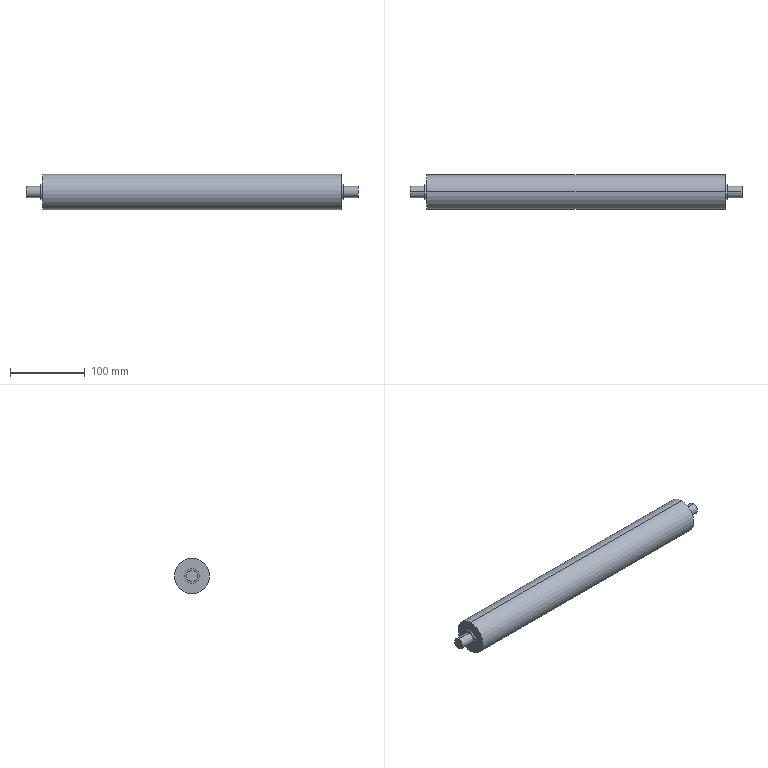Part | SolidWorks | features Revolution 1 | 1 solid | 16 faces | box 445 x 47 x 47 mm | volume 702617 mm3 | cylinder 10 | plane 6 | commonest cylinder face diameters 15 x4 20 x4 47 x2
STEP:
#1=CARTESIAN_POINT('',(425.,0.,-7.5));
#2=VERTEX_POINT('',#1);
#3=CARTESIAN_POINT('',(425.,0.,7.5));
#4=VERTEX_POINT('',#3);
#5=CARTESIAN_POINT('',(425.,0.,0.));
#6=DIRECTION('',(1.,0.,0.));
#7=DIRECTION('',(0.,0.,-1.));
#8=AXIS2_PLACEMENT_3D('',#5,#6,#7);
#9=CIRCLE('',#8,7.5);
#10=EDGE_CURVE('',#2,#4,#9,.T.);
#11=ORIENTED_EDGE('',*,*,#10,.T.);
#12=CARTESIAN_POINT('',(445.,0.,7.5));
#13=VERTEX_POINT('',#12);
#14=CARTESIAN_POINT('',(0.,0.,7.5));
#15=DIRECTION('',(1.,0.,0.));
#16=VECTOR('',#15,1000.);
#17=LINE('',#14,#16);
#18=EDGE_CURVE('',#4,#13,#17,.T.);
#19=ORIENTED_EDGE('',*,*,#18,.T.);
#20=CARTESIAN_POINT('',(445.,0.,-7.5));
#21=VERTEX_POINT('',#20);
#22=CARTESIAN_POINT('',(445.,0.,0.));
#23=DIRECTION('',(1.,0.,0.));
#24=DIRECTION('',(0.,0.,-1.));
#25=AXIS2_PLACEMENT_3D('',#22,#23,#24);
#26=CIRCLE('',#25,7.5);
#27=EDGE_CURVE('',#21,#13,#26,.T.);
#28=ORIENTED_EDGE('',*,*,#27,.F.);
#29=CARTESIAN_POINT('',(0.,0.,-7.5));
#30=DIRECTION('',(1.,0.,0.));
#31=VECTOR('',#30,1000.);
#32=LINE('',#29,#31);
#33=EDGE_CURVE('',#2,#21,#32,.T.);
#34=ORIENTED_EDGE('',*,*,#33,.F.);
#35=EDGE_LOOP('',(#11,#19,#28,#34));
#36=FACE_OUTER_BOUND('',#35,.T.);
#37=CARTESIAN_POINT('',(0.,0.,0.));
#38=DIRECTION('',(1.,0.,0.));
#39=DIRECTION('',(0.,0.,-1.));
#40=AXIS2_PLACEMENT_3D('',#37,#38,#39);
#41=CYLINDRICAL_SURFACE('',#40,7.5);
#42=ADVANCED_FACE('',(#36),#41,.T.);
#43=CARTESIAN_POINT('',(422.5,0.,-10.));
#44=VERTEX_POINT('',#43);
#45=CARTESIAN_POINT('',(422.5,0.,10.));
#46=VERTEX_POINT('',#45);
#47=CARTESIAN_POINT('',(422.5,0.,0.));
#48=DIRECTION('',(1.,0.,0.));
#49=DIRECTION('',(0.,0.,-1.));
#50=AXIS2_PLACEMENT_3D('',#47,#48,#49);
#51=CIRCLE('',#50,10.);
#52=EDGE_CURVE('',#44,#46,#51,.T.);
#53=ORIENTED_EDGE('',*,*,#52,.T.);
#54=CARTESIAN_POINT('',(425.,0.,10.));
#55=VERTEX_POINT('',#54);
#56=CARTESIAN_POINT('',(0.,0.,10.));
#57=DIRECTION('',(1.,0.,0.));
#58=VECTOR('',#57,1000.);
#59=LINE('',#56,#58);
#60=EDGE_CURVE('',#46,#55,#59,.T.);
#61=ORIENTED_EDGE('',*,*,#60,.T.);
#62=CARTESIAN_POINT('',(425.,0.,-10.));
#63=VERTEX_POINT('',#62);
#64=CARTESIAN_POINT('',(425.,0.,0.));
#65=DIRECTION('',(1.,0.,0.));
#66=DIRECTION('',(0.,0.,-1.));
#67=AXIS2_PLACEMENT_3D('',#64,#65,#66);
#68=CIRCLE('',#67,10.);
#69=EDGE_CURVE('',#63,#55,#68,.T.);
#70=ORIENTED_EDGE('',*,*,#69,.F.);
#71=CARTESIAN_POINT('',(0.,0.,-10.));
#72=DIRECTION('',(1.,0.,0.));
#73=VECTOR('',#72,1000.);
#74=LINE('',#71,#73);
#75=EDGE_CURVE('',#44,#63,#74,.T.);
#76=ORIENTED_EDGE('',*,*,#75,.F.);
#77=EDGE_LOOP('',(#53,#61,#70,#76));
#78=FACE_OUTER_BOUND('',#77,.T.);
#79=CARTESIAN_POINT('',(0.,0.,0.));
#80=DIRECTION('',(1.,0.,0.));
#81=DIRECTION('',(0.,0.,-1.));
#82=AXIS2_PLACEMENT_3D('',#79,#80,#81);
#83=CYLINDRICAL_SURFACE('',#82,10.);
#84=ADVANCED_FACE('',(#78),#83,.T.);
#85=CARTESIAN_POINT('',(22.5,0.,-23.5));
#86=VERTEX_POINT('',#85);
#87=CARTESIAN_POINT('',(22.5,0.,23.5));
#88=VERTEX_POINT('',#87);
#89=CARTESIAN_POINT('',(22.5,0.,0.));
#90=DIRECTION('',(1.,0.,0.));
#91=DIRECTION('',(0.,0.,-1.));
#92=AXIS2_PLACEMENT_3D('',#89,#90,#91);
#93=CIRCLE('',#92,23.5);
#94=EDGE_CURVE('',#86,#88,#93,.T.);
#95=ORIENTED_EDGE('',*,*,#94,.T.);
#96=CARTESIAN_POINT('',(422.5,0.,23.5));
#97=VERTEX_POINT('',#96);
#98=CARTESIAN_POINT('',(0.,0.,23.5));
#99=DIRECTION('',(1.,0.,0.));
#100=VECTOR('',#99,1000.);
#101=LINE('',#98,#100);
#102=EDGE_CURVE('',#88,#97,#101,.T.);
#103=ORIENTED_EDGE('',*,*,#102,.T.);
#104=CARTESIAN_POINT('',(422.5,0.,-23.5));
#105=VERTEX_POINT('',#104);
#106=CARTESIAN_POINT('',(422.5,0.,0.));
#107=DIRECTION('',(1.,0.,0.));
#108=DIRECTION('',(0.,0.,-1.));
#109=AXIS2_PLACEMENT_3D('',#106,#107,#108);
#110=CIRCLE('',#109,23.5);
#111=EDGE_CURVE('',#105,#97,#110,.T.);
#112=ORIENTED_EDGE('',*,*,#111,.F.);
#113=CARTESIAN_POINT('',(0.,0.,-23.5));
#114=DIRECTION('',(1.,0.,0.));
#115=VECTOR('',#114,1000.);
#116=LINE('',#113,#115);
#117=EDGE_CURVE('',#86,#105,#116,.T.);
#118=ORIENTED_EDGE('',*,*,#117,.F.);
#119=EDGE_LOOP('',(#95,#103,#112,#118));
#120=FACE_OUTER_BOUND('',#119,.T.);
#121=CARTESIAN_POINT('',(0.,0.,0.));
#122=DIRECTION('',(1.,0.,0.));
#123=DIRECTION('',(0.,0.,-1.));
#124=AXIS2_PLACEMENT_3D('',#121,#122,#123);
#125=CYLINDRICAL_SURFACE('',#124,23.5);
#126=ADVANCED_FACE('',(#120),#125,.T.);
#127=CARTESIAN_POINT('',(20.,0.,-10.));
#128=VERTEX_POINT('',#127);
#129=CARTESIAN_POINT('',(20.,0.,10.));
#130=VERTEX_POINT('',#129);
#131=CARTESIAN_POINT('',(20.,0.,0.));
#132=DIRECTION('',(1.,0.,0.));
#133=DIRECTION('',(0.,0.,-1.));
#134=AXIS2_PLACEMENT_3D('',#131,#132,#133);
#135=CIRCLE('',#134,10.);
#136=EDGE_CURVE('',#128,#130,#135,.T.);
#137=ORIENTED_EDGE('',*,*,#136,.T.);
#138=CARTESIAN_POINT('',(22.5,0.,10.));
#139=VERTEX_POINT('',#138);
#140=CARTESIAN_POINT('',(0.,0.,10.));
#141=DIRECTION('',(1.,0.,0.));
#142=VECTOR('',#141,1000.);
#143=LINE('',#140,#142);
#144=EDGE_CURVE('',#130,#139,#143,.T.);
#145=ORIENTED_EDGE('',*,*,#144,.T.);
#146=CARTESIAN_POINT('',(22.5,0.,-10.));
#147=VERTEX_POINT('',#146);
#148=CARTESIAN_POINT('',(22.5,0.,0.));
#149=DIRECTION('',(1.,0.,0.));
#150=DIRECTION('',(0.,0.,-1.));
#151=AXIS2_PLACEMENT_3D('',#148,#149,#150);
#152=CIRCLE('',#151,10.);
#153=EDGE_CURVE('',#147,#139,#152,.T.);
#154=ORIENTED_EDGE('',*,*,#153,.F.);
#155=CARTESIAN_POINT('',(0.,0.,-10.));
#156=DIRECTION('',(1.,0.,0.));
#157=VECTOR('',#156,1000.);
#158=LINE('',#155,#157);
#159=EDGE_CURVE('',#128,#147,#158,.T.);
#160=ORIENTED_EDGE('',*,*,#159,.F.);
#161=EDGE_LOOP('',(#137,#145,#154,#160));
#162=FACE_OUTER_BOUND('',#161,.T.);
#163=CARTESIAN_POINT('',(0.,0.,0.));
#164=DIRECTION('',(1.,0.,0.));
#165=DIRECTION('',(0.,0.,-1.));
#166=AXIS2_PLACEMENT_3D('',#163,#164,#165);
#167=CYLINDRICAL_SURFACE('',#166,10.);
#168=ADVANCED_FACE('',(#162),#167,.T.);
#169=CARTESIAN_POINT('',(0.,0.,-7.5));
#170=VERTEX_POINT('',#169);
#171=CARTESIAN_POINT('',(0.,0.,7.5));
#172=VERTEX_POINT('',#171);
#173=CARTESIAN_POINT('',(0.,0.,0.));
#174=DIRECTION('',(1.,0.,0.));
#175=DIRECTION('',(0.,0.,-1.));
#176=AXIS2_PLACEMENT_3D('',#173,#174,#175);
#177=CIRCLE('',#176,7.5);
#178=EDGE_CURVE('',#170,#172,#177,.T.);
#179=ORIENTED_EDGE('',*,*,#178,.T.);
#180=CARTESIAN_POINT('',(20.,0.,7.5));
#181=VERTEX_POINT('',#180);
#182=CARTESIAN_POINT('',(0.,0.,7.5));
#183=DIRECTION('',(1.,0.,0.));
#184=VECTOR('',#183,1000.);
#185=LINE('',#182,#184);
#186=EDGE_CURVE('',#172,#181,#185,.T.);
#187=ORIENTED_EDGE('',*,*,#186,.T.);
#188=CARTESIAN_POINT('',(20.,0.,-7.5));
#189=VERTEX_POINT('',#188);
#190=CARTESIAN_POINT('',(20.,0.,0.));
#191=DIRECTION('',(1.,0.,0.));
#192=DIRECTION('',(0.,0.,-1.));
#193=AXIS2_PLACEMENT_3D('',#190,#191,#192);
#194=CIRCLE('',#193,7.5);
#195=EDGE_CURVE('',#189,#181,#194,.T.);
#196=ORIENTED_EDGE('',*,*,#195,.F.);
#197=CARTESIAN_POINT('',(0.,0.,-7.5));
#198=DIRECTION('',(1.,0.,0.));
#199=VECTOR('',#198,1000.);
#200=LINE('',#197,#199);
#201=EDGE_CURVE('',#170,#189,#200,.T.);
#202=ORIENTED_EDGE('',*,*,#201,.F.);
#203=EDGE_LOOP('',(#179,#187,#196,#202));
#204=FACE_OUTER_BOUND('',#203,.T.);
#205=CARTESIAN_POINT('',(0.,0.,0.));
#206=DIRECTION('',(1.,0.,0.));
#207=DIRECTION('',(0.,0.,-1.));
#208=AXIS2_PLACEMENT_3D('',#205,#206,#207);
#209=CYLINDRICAL_SURFACE('',#208,7.5);
#210=ADVANCED_FACE('',(#204),#209,.T.);
#211=ORIENTED_EDGE('',*,*,#178,.F.);
#212=CARTESIAN_POINT('',(0.,0.,0.));
#213=DIRECTION('',(1.,0.,0.));
#214=DIRECTION('',(0.,0.,-1.));
#215=AXIS2_PLACEMENT_3D('',#212,#213,#214);
#216=CIRCLE('',#215,7.5);
#217=EDGE_CURVE('',#172,#170,#216,.T.);
#218=ORIENTED_EDGE('',*,*,#217,.F.);
#219=EDGE_LOOP('',(#211,#218));
#220=FACE_OUTER_BOUND('',#219,.T.);
#221=CARTESIAN_POINT('',(0.,0.,0.));
#222=DIRECTION('',(-1.,0.,0.));
#223=DIRECTION('',(0.,0.,1.));
#224=AXIS2_PLACEMENT_3D('',#221,#222,#223);
#225=PLANE('',#224);
#226=ADVANCED_FACE('',(#220),#225,.T.);
#227=ORIENTED_EDGE('',*,*,#186,.F.);
#228=ORIENTED_EDGE('',*,*,#217,.T.);
#229=ORIENTED_EDGE('',*,*,#201,.T.);
#230=CARTESIAN_POINT('',(20.,0.,0.));
#231=DIRECTION('',(1.,0.,0.));
#232=DIRECTION('',(0.,0.,-1.));
#233=AXIS2_PLACEMENT_3D('',#230,#231,#232);
#234=CIRCLE('',#233,7.5);
#235=EDGE_CURVE('',#181,#189,#234,.T.);
#236=ORIENTED_EDGE('',*,*,#235,.F.);
#237=EDGE_LOOP('',(#227,#228,#229,#236));
#238=FACE_OUTER_BOUND('',#237,.T.);
#239=CARTESIAN_POINT('',(0.,0.,0.));
#240=DIRECTION('',(1.,0.,0.));
#241=DIRECTION('',(0.,0.,-1.));
#242=AXIS2_PLACEMENT_3D('',#239,#240,#241);
#243=CYLINDRICAL_SURFACE('',#242,7.5);
#244=ADVANCED_FACE('',(#238),#243,.T.);
#245=ORIENTED_EDGE('',*,*,#195,.T.);
#246=ORIENTED_EDGE('',*,*,#235,.T.);
#247=EDGE_LOOP('',(#245,#246));
#248=FACE_BOUND('',#247,.T.);
#249=ORIENTED_EDGE('',*,*,#136,.F.);
#250=CARTESIAN_POINT('',(20.,0.,0.));
#251=DIRECTION('',(1.,0.,0.));
#252=DIRECTION('',(0.,0.,-1.));
#253=AXIS2_PLACEMENT_3D('',#250,#251,#252);
#254=CIRCLE('',#253,10.);
#255=EDGE_CURVE('',#130,#128,#254,.T.);
#256=ORIENTED_EDGE('',*,*,#255,.F.);
#257=EDGE_LOOP('',(#249,#256));
#258=FACE_OUTER_BOUND('',#257,.T.);
#259=CARTESIAN_POINT('',(20.,7.5,0.));
#260=DIRECTION('',(-1.,0.,0.));
#261=DIRECTION('',(0.,0.,1.));
#262=AXIS2_PLACEMENT_3D('',#259,#260,#261);
#263=PLANE('',#262);
#264=ADVANCED_FACE('',(#248,#258),#263,.T.);
#265=ORIENTED_EDGE('',*,*,#144,.F.);
#266=ORIENTED_EDGE('',*,*,#255,.T.);
#267=ORIENTED_EDGE('',*,*,#159,.T.);
#268=CARTESIAN_POINT('',(22.5,0.,0.));
#269=DIRECTION('',(1.,0.,0.));
#270=DIRECTION('',(0.,0.,-1.));
#271=AXIS2_PLACEMENT_3D('',#268,#269,#270);
#272=CIRCLE('',#271,10.);
#273=EDGE_CURVE('',#139,#147,#272,.T.);
#274=ORIENTED_EDGE('',*,*,#273,.F.);
#275=EDGE_LOOP('',(#265,#266,#267,#274));
#276=FACE_OUTER_BOUND('',#275,.T.);
#277=CARTESIAN_POINT('',(0.,0.,0.));
#278=DIRECTION('',(1.,0.,0.));
#279=DIRECTION('',(0.,0.,-1.));
#280=AXIS2_PLACEMENT_3D('',#277,#278,#279);
#281=CYLINDRICAL_SURFACE('',#280,10.);
#282=ADVANCED_FACE('',(#276),#281,.T.);
#283=ORIENTED_EDGE('',*,*,#153,.T.);
#284=ORIENTED_EDGE('',*,*,#273,.T.);
#285=EDGE_LOOP('',(#283,#284));
#286=FACE_BOUND('',#285,.T.);
#287=ORIENTED_EDGE('',*,*,#94,.F.);
#288=CARTESIAN_POINT('',(22.5,0.,0.));
#289=DIRECTION('',(1.,0.,0.));
#290=DIRECTION('',(0.,0.,-1.));
#291=AXIS2_PLACEMENT_3D('',#288,#289,#290);
#292=CIRCLE('',#291,23.5);
#293=EDGE_CURVE('',#88,#86,#292,.T.);
#294=ORIENTED_EDGE('',*,*,#293,.F.);
#295=EDGE_LOOP('',(#287,#294));
#296=FACE_OUTER_BOUND('',#295,.T.);
#297=CARTESIAN_POINT('',(22.5,10.,0.));
#298=DIRECTION('',(-1.,0.,0.));
#299=DIRECTION('',(0.,0.,1.));
#300=AXIS2_PLACEMENT_3D('',#297,#298,#299);
#301=PLANE('',#300);
#302=ADVANCED_FACE('',(#286,#296),#301,.T.);
#303=ORIENTED_EDGE('',*,*,#102,.F.);
#304=ORIENTED_EDGE('',*,*,#293,.T.);
#305=ORIENTED_EDGE('',*,*,#117,.T.);
#306=CARTESIAN_POINT('',(422.5,0.,0.));
#307=DIRECTION('',(1.,0.,0.));
#308=DIRECTION('',(0.,0.,-1.));
#309=AXIS2_PLACEMENT_3D('',#306,#307,#308);
#310=CIRCLE('',#309,23.5);
#311=EDGE_CURVE('',#97,#105,#310,.T.);
#312=ORIENTED_EDGE('',*,*,#311,.F.);
#313=EDGE_LOOP('',(#303,#304,#305,#312));
#314=FACE_OUTER_BOUND('',#313,.T.);
#315=CARTESIAN_POINT('',(0.,0.,0.));
#316=DIRECTION('',(1.,0.,0.));
#317=DIRECTION('',(0.,0.,-1.));
#318=AXIS2_PLACEMENT_3D('',#315,#316,#317);
#319=CYLINDRICAL_SURFACE('',#318,23.5);
#320=ADVANCED_FACE('',(#314),#319,.T.);
#321=ORIENTED_EDGE('',*,*,#111,.T.);
#322=ORIENTED_EDGE('',*,*,#311,.T.);
#323=EDGE_LOOP('',(#321,#322));
#324=FACE_OUTER_BOUND('',#323,.T.);
#325=ORIENTED_EDGE('',*,*,#52,.F.);
#326=CARTESIAN_POINT('',(422.5,0.,0.));
#327=DIRECTION('',(1.,0.,0.));
#328=DIRECTION('',(0.,0.,-1.));
#329=AXIS2_PLACEMENT_3D('',#326,#327,#328);
#330=CIRCLE('',#329,10.);
#331=EDGE_CURVE('',#46,#44,#330,.T.);
#332=ORIENTED_EDGE('',*,*,#331,.F.);
#333=EDGE_LOOP('',(#325,#332));
#334=FACE_BOUND('',#333,.T.);
#335=CARTESIAN_POINT('',(422.5,10.,0.));
#336=DIRECTION('',(1.,0.,0.));
#337=DIRECTION('',(0.,0.,-1.));
#338=AXIS2_PLACEMENT_3D('',#335,#336,#337);
#339=PLANE('',#338);
#340=ADVANCED_FACE('',(#324,#334),#339,.T.);
#341=ORIENTED_EDGE('',*,*,#60,.F.);
#342=ORIENTED_EDGE('',*,*,#331,.T.);
#343=ORIENTED_EDGE('',*,*,#75,.T.);
#344=CARTESIAN_POINT('',(425.,0.,0.));
#345=DIRECTION('',(1.,0.,0.));
#346=DIRECTION('',(0.,0.,-1.));
#347=AXIS2_PLACEMENT_3D('',#344,#345,#346);
#348=CIRCLE('',#347,10.);
#349=EDGE_CURVE('',#55,#63,#348,.T.);
#350=ORIENTED_EDGE('',*,*,#349,.F.);
#351=EDGE_LOOP('',(#341,#342,#343,#350));
#352=FACE_OUTER_BOUND('',#351,.T.);
#353=CARTESIAN_POINT('',(0.,0.,0.));
#354=DIRECTION('',(1.,0.,0.));
#355=DIRECTION('',(0.,0.,-1.));
#356=AXIS2_PLACEMENT_3D('',#353,#354,#355);
#357=CYLINDRICAL_SURFACE('',#356,10.);
#358=ADVANCED_FACE('',(#352),#357,.T.);
#359=ORIENTED_EDGE('',*,*,#69,.T.);
#360=ORIENTED_EDGE('',*,*,#349,.T.);
#361=EDGE_LOOP('',(#359,#360));
#362=FACE_OUTER_BOUND('',#361,.T.);
#363=ORIENTED_EDGE('',*,*,#10,.F.);
#364=CARTESIAN_POINT('',(425.,0.,0.));
#365=DIRECTION('',(1.,0.,0.));
#366=DIRECTION('',(0.,0.,-1.));
#367=AXIS2_PLACEMENT_3D('',#364,#365,#366);
#368=CIRCLE('',#367,7.5);
#369=EDGE_CURVE('',#4,#2,#368,.T.);
#370=ORIENTED_EDGE('',*,*,#369,.F.);
#371=EDGE_LOOP('',(#363,#370));
#372=FACE_BOUND('',#371,.T.);
#373=CARTESIAN_POINT('',(425.,7.5,0.));
#374=DIRECTION('',(1.,0.,0.));
#375=DIRECTION('',(0.,0.,-1.));
#376=AXIS2_PLACEMENT_3D('',#373,#374,#375);
#377=PLANE('',#376);
#378=ADVANCED_FACE('',(#362,#372),#377,.T.);
#379=ORIENTED_EDGE('',*,*,#18,.F.);
#380=ORIENTED_EDGE('',*,*,#369,.T.);
#381=ORIENTED_EDGE('',*,*,#33,.T.);
#382=CARTESIAN_POINT('',(445.,0.,0.));
#383=DIRECTION('',(1.,0.,0.));
#384=DIRECTION('',(0.,0.,-1.));
#385=AXIS2_PLACEMENT_3D('',#382,#383,#384);
#386=CIRCLE('',#385,7.5);
#387=EDGE_CURVE('',#13,#21,#386,.T.);
#388=ORIENTED_EDGE('',*,*,#387,.F.);
#389=EDGE_LOOP('',(#379,#380,#381,#388));
#390=FACE_OUTER_BOUND('',#389,.T.);
#391=CARTESIAN_POINT('',(0.,0.,0.));
#392=DIRECTION('',(1.,0.,0.));
#393=DIRECTION('',(0.,0.,-1.));
#394=AXIS2_PLACEMENT_3D('',#391,#392,#393);
#395=CYLINDRICAL_SURFACE('',#394,7.5);
#396=ADVANCED_FACE('',(#390),#395,.T.);
#397=ORIENTED_EDGE('',*,*,#27,.T.);
#398=ORIENTED_EDGE('',*,*,#387,.T.);
#399=EDGE_LOOP('',(#397,#398));
#400=FACE_OUTER_BOUND('',#399,.T.);
#401=CARTESIAN_POINT('',(445.,0.,0.));
#402=DIRECTION('',(1.,0.,0.));
#403=DIRECTION('',(0.,0.,-1.));
#404=AXIS2_PLACEMENT_3D('',#401,#402,#403);
#405=PLANE('',#404);
#406=ADVANCED_FACE('',(#400),#405,.T.);
#407=CLOSED_SHELL('',(#42,#84,#126,#168,#210,#226,#244,#264,#282,#302,#320,#340,#358,#378,#396,#406));
#408=MANIFOLD_SOLID_BREP('',#407);
#409=CARTESIAN_POINT('',(0.,0.,0.));
#410=DIRECTION('',(0.,0.,1.));
#411=DIRECTION('',(1.,0.,0.));
#412=AXIS2_PLACEMENT_3D('',#409,#410,#411);
#413=(LENGTH_UNIT()NAMED_UNIT(*)SI_UNIT(.MILLI.,.METRE.));
#414=UNCERTAINTY_MEASURE_WITH_UNIT(LENGTH_MEASURE(0.00001),#413,'','');
#415=(NAMED_UNIT(*)PLANE_ANGLE_UNIT()SI_UNIT($,.RADIAN.));
#416=(NAMED_UNIT(*)SI_UNIT($,.STERADIAN.)SOLID_ANGLE_UNIT());
#417=(GEOMETRIC_REPRESENTATION_CONTEXT(3)GLOBAL_UNCERTAINTY_ASSIGNED_CONTEXT((#414))GLOBAL_UNIT_ASSIGNED_CONTEXT((#413,#415,#416))REPRESENTATION_CONTEXT('',''));
#418=ADVANCED_BREP_SHAPE_REPRESENTATION('',(#408,#412),#417);